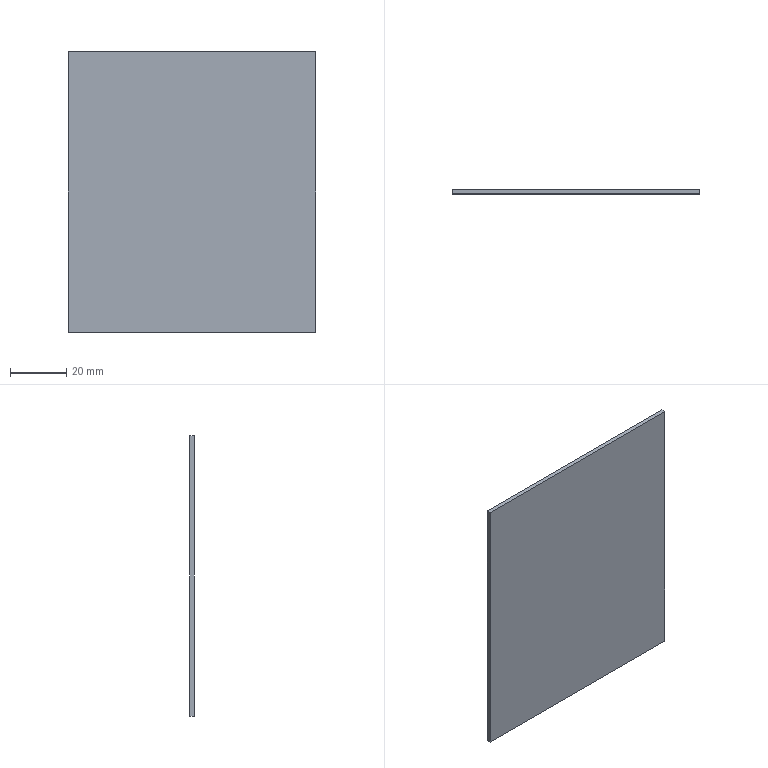Part | STEP file | 1 solid | 6 faces | box 88 x 1.5 x 100 mm | volume 13200 mm3 | plane 6
STEP:
#1=CARTESIAN_POINT('',(0.,0.,0.));
#2=DIRECTION('',(0.,0.,1.));
#3=DIRECTION('',(1.,0.,0.));
#4=AXIS2_PLACEMENT_3D('',#1,#2,#3);
#5=CARTESIAN_POINT('',(44.,0.,50.));
#6=VERTEX_POINT('',#5);
#7=CARTESIAN_POINT('',(44.,0.,-50.));
#8=VERTEX_POINT('',#7);
#9=CARTESIAN_POINT('',(44.,0.,-50.));
#10=DIRECTION('',(0.,0.,-1.));
#11=VECTOR('',#10,1.);
#12=LINE('',#9,#11);
#13=CARTESIAN_POINT('',(44.,1.5,-50.));
#14=DIRECTION('',(-1.,0.,0.));
#15=DIRECTION('',(0.,0.,1.));
#16=AXIS2_PLACEMENT_3D('',#13,#14,#15);
#17=PLANE('',#16);
#18=CARTESIAN_POINT('',(0.,-1.5));
#19=DIRECTION('',(-1.,0.));
#20=VECTOR('',#19,1.);
#21=LINE('',#18,#20);
#22=(GEOMETRIC_REPRESENTATION_CONTEXT(2)PARAMETRIC_REPRESENTATION_CONTEXT()REPRESENTATION_CONTEXT('',''));
#23=DEFINITIONAL_REPRESENTATION('',(#21),#22);
#24=PCURVE('',#17,#23);
#25=CARTESIAN_POINT('',(0.,0.,0.));
#26=DIRECTION('',(0.,1.,0.));
#27=DIRECTION('',(0.,0.,1.));
#28=AXIS2_PLACEMENT_3D('',#25,#26,#27);
#29=PLANE('',#28);
#30=CARTESIAN_POINT('',(-50.,44.));
#31=DIRECTION('',(-1.,0.));
#32=VECTOR('',#31,1.);
#33=LINE('',#30,#32);
#34=(GEOMETRIC_REPRESENTATION_CONTEXT(2)PARAMETRIC_REPRESENTATION_CONTEXT()REPRESENTATION_CONTEXT('',''));
#35=DEFINITIONAL_REPRESENTATION('',(#33),#34);
#36=PCURVE('',#29,#35);
#37=SURFACE_CURVE('',#12,(#24,#36),.PCURVE_S1.);
#38=EDGE_CURVE('',#6,#8,#37,.T.);
#39=ORIENTED_EDGE('',*,*,#38,.T.);
#40=CARTESIAN_POINT('',(44.,1.5,-50.));
#41=VERTEX_POINT('',#40);
#42=CARTESIAN_POINT('',(44.,1.5,-50.));
#43=DIRECTION('',(0.,-1.,0.));
#44=VECTOR('',#43,1.);
#45=LINE('',#42,#44);
#46=CARTESIAN_POINT('',(0.,0.));
#47=DIRECTION('',(0.,-1.));
#48=VECTOR('',#47,1.);
#49=LINE('',#46,#48);
#50=(GEOMETRIC_REPRESENTATION_CONTEXT(2)PARAMETRIC_REPRESENTATION_CONTEXT()REPRESENTATION_CONTEXT('',''));
#51=DEFINITIONAL_REPRESENTATION('',(#49),#50);
#52=PCURVE('',#17,#51);
#53=CARTESIAN_POINT('',(-44.,1.5,-50.));
#54=DIRECTION('',(0.,0.,1.));
#55=DIRECTION('',(1.,0.,0.));
#56=AXIS2_PLACEMENT_3D('',#53,#54,#55);
#57=PLANE('',#56);
#58=CARTESIAN_POINT('',(88.,0.));
#59=DIRECTION('',(0.,-1.));
#60=VECTOR('',#59,1.);
#61=LINE('',#58,#60);
#62=(GEOMETRIC_REPRESENTATION_CONTEXT(2)PARAMETRIC_REPRESENTATION_CONTEXT()REPRESENTATION_CONTEXT('',''));
#63=DEFINITIONAL_REPRESENTATION('',(#61),#62);
#64=PCURVE('',#57,#63);
#65=SURFACE_CURVE('',#45,(#52,#64),.PCURVE_S1.);
#66=EDGE_CURVE('',#41,#8,#65,.T.);
#67=ORIENTED_EDGE('',*,*,#66,.F.);
#68=CARTESIAN_POINT('',(44.,1.5,50.));
#69=VERTEX_POINT('',#68);
#70=CARTESIAN_POINT('',(44.,1.5,-50.));
#71=DIRECTION('',(0.,0.,-1.));
#72=VECTOR('',#71,1.);
#73=LINE('',#70,#72);
#74=CARTESIAN_POINT('',(0.,0.));
#75=DIRECTION('',(-1.,0.));
#76=VECTOR('',#75,1.);
#77=LINE('',#74,#76);
#78=(GEOMETRIC_REPRESENTATION_CONTEXT(2)PARAMETRIC_REPRESENTATION_CONTEXT()REPRESENTATION_CONTEXT('',''));
#79=DEFINITIONAL_REPRESENTATION('',(#77),#78);
#80=PCURVE('',#17,#79);
#81=CARTESIAN_POINT('',(0.,1.5,0.));
#82=DIRECTION('',(0.,1.,0.));
#83=DIRECTION('',(0.,0.,1.));
#84=AXIS2_PLACEMENT_3D('',#81,#82,#83);
#85=PLANE('',#84);
#86=CARTESIAN_POINT('',(-50.,44.));
#87=DIRECTION('',(-1.,0.));
#88=VECTOR('',#87,1.);
#89=LINE('',#86,#88);
#90=(GEOMETRIC_REPRESENTATION_CONTEXT(2)PARAMETRIC_REPRESENTATION_CONTEXT()REPRESENTATION_CONTEXT('',''));
#91=DEFINITIONAL_REPRESENTATION('',(#89),#90);
#92=PCURVE('',#85,#91);
#93=SURFACE_CURVE('',#73,(#80,#92),.PCURVE_S1.);
#94=EDGE_CURVE('',#69,#41,#93,.T.);
#95=ORIENTED_EDGE('',*,*,#94,.F.);
#96=CARTESIAN_POINT('',(44.,1.5,50.));
#97=DIRECTION('',(0.,-1.,0.));
#98=VECTOR('',#97,1.);
#99=LINE('',#96,#98);
#100=CARTESIAN_POINT('',(100.,0.));
#101=DIRECTION('',(0.,-1.));
#102=VECTOR('',#101,1.);
#103=LINE('',#100,#102);
#104=(GEOMETRIC_REPRESENTATION_CONTEXT(2)PARAMETRIC_REPRESENTATION_CONTEXT()REPRESENTATION_CONTEXT('',''));
#105=DEFINITIONAL_REPRESENTATION('',(#103),#104);
#106=PCURVE('',#17,#105);
#107=CARTESIAN_POINT('',(-44.,1.5,50.));
#108=DIRECTION('',(0.,0.,-1.));
#109=DIRECTION('',(-1.,0.,0.));
#110=AXIS2_PLACEMENT_3D('',#107,#108,#109);
#111=PLANE('',#110);
#112=CARTESIAN_POINT('',(-88.,0.));
#113=DIRECTION('',(0.,-1.));
#114=VECTOR('',#113,1.);
#115=LINE('',#112,#114);
#116=(GEOMETRIC_REPRESENTATION_CONTEXT(2)PARAMETRIC_REPRESENTATION_CONTEXT()REPRESENTATION_CONTEXT('',''));
#117=DEFINITIONAL_REPRESENTATION('',(#115),#116);
#118=PCURVE('',#111,#117);
#119=SURFACE_CURVE('',#99,(#106,#118),.PCURVE_S1.);
#120=EDGE_CURVE('',#69,#6,#119,.T.);
#121=ORIENTED_EDGE('',*,*,#120,.T.);
#122=EDGE_LOOP('',(#39,#67,#95,#121));
#123=FACE_BOUND('',#122,.T.);
#124=ADVANCED_FACE('',(#123),#17,.F.);
#125=CARTESIAN_POINT('',(-44.,0.,-50.));
#126=VERTEX_POINT('',#125);
#127=CARTESIAN_POINT('',(-44.,0.,-50.));
#128=DIRECTION('',(-1.,0.,0.));
#129=VECTOR('',#128,1.);
#130=LINE('',#127,#129);
#131=CARTESIAN_POINT('',(0.,-1.5));
#132=DIRECTION('',(-1.,0.));
#133=VECTOR('',#132,1.);
#134=LINE('',#131,#133);
#135=(GEOMETRIC_REPRESENTATION_CONTEXT(2)PARAMETRIC_REPRESENTATION_CONTEXT()REPRESENTATION_CONTEXT('',''));
#136=DEFINITIONAL_REPRESENTATION('',(#134),#135);
#137=PCURVE('',#57,#136);
#138=CARTESIAN_POINT('',(-50.,-44.));
#139=DIRECTION('',(0.,-1.));
#140=VECTOR('',#139,1.);
#141=LINE('',#138,#140);
#142=(GEOMETRIC_REPRESENTATION_CONTEXT(2)PARAMETRIC_REPRESENTATION_CONTEXT()REPRESENTATION_CONTEXT('',''));
#143=DEFINITIONAL_REPRESENTATION('',(#141),#142);
#144=PCURVE('',#29,#143);
#145=SURFACE_CURVE('',#130,(#137,#144),.PCURVE_S1.);
#146=EDGE_CURVE('',#8,#126,#145,.T.);
#147=ORIENTED_EDGE('',*,*,#146,.T.);
#148=CARTESIAN_POINT('',(-44.,1.5,-50.));
#149=VERTEX_POINT('',#148);
#150=CARTESIAN_POINT('',(-44.,1.5,-50.));
#151=DIRECTION('',(0.,-1.,0.));
#152=VECTOR('',#151,1.);
#153=LINE('',#150,#152);
#154=CARTESIAN_POINT('',(0.,0.));
#155=DIRECTION('',(0.,-1.));
#156=VECTOR('',#155,1.);
#157=LINE('',#154,#156);
#158=(GEOMETRIC_REPRESENTATION_CONTEXT(2)PARAMETRIC_REPRESENTATION_CONTEXT()REPRESENTATION_CONTEXT('',''));
#159=DEFINITIONAL_REPRESENTATION('',(#157),#158);
#160=PCURVE('',#57,#159);
#161=CARTESIAN_POINT('',(-44.,1.5,-50.));
#162=DIRECTION('',(1.,0.,0.));
#163=DIRECTION('',(0.,0.,-1.));
#164=AXIS2_PLACEMENT_3D('',#161,#162,#163);
#165=PLANE('',#164);
#166=CARTESIAN_POINT('',(0.,0.));
#167=DIRECTION('',(0.,-1.));
#168=VECTOR('',#167,1.);
#169=LINE('',#166,#168);
#170=(GEOMETRIC_REPRESENTATION_CONTEXT(2)PARAMETRIC_REPRESENTATION_CONTEXT()REPRESENTATION_CONTEXT('',''));
#171=DEFINITIONAL_REPRESENTATION('',(#169),#170);
#172=PCURVE('',#165,#171);
#173=SURFACE_CURVE('',#153,(#160,#172),.PCURVE_S1.);
#174=EDGE_CURVE('',#149,#126,#173,.T.);
#175=ORIENTED_EDGE('',*,*,#174,.F.);
#176=CARTESIAN_POINT('',(-44.,1.5,-50.));
#177=DIRECTION('',(-1.,0.,0.));
#178=VECTOR('',#177,1.);
#179=LINE('',#176,#178);
#180=CARTESIAN_POINT('',(0.,0.));
#181=DIRECTION('',(-1.,0.));
#182=VECTOR('',#181,1.);
#183=LINE('',#180,#182);
#184=(GEOMETRIC_REPRESENTATION_CONTEXT(2)PARAMETRIC_REPRESENTATION_CONTEXT()REPRESENTATION_CONTEXT('',''));
#185=DEFINITIONAL_REPRESENTATION('',(#183),#184);
#186=PCURVE('',#57,#185);
#187=CARTESIAN_POINT('',(-50.,-44.));
#188=DIRECTION('',(0.,-1.));
#189=VECTOR('',#188,1.);
#190=LINE('',#187,#189);
#191=(GEOMETRIC_REPRESENTATION_CONTEXT(2)PARAMETRIC_REPRESENTATION_CONTEXT()REPRESENTATION_CONTEXT('',''));
#192=DEFINITIONAL_REPRESENTATION('',(#190),#191);
#193=PCURVE('',#85,#192);
#194=SURFACE_CURVE('',#179,(#186,#193),.PCURVE_S1.);
#195=EDGE_CURVE('',#41,#149,#194,.T.);
#196=ORIENTED_EDGE('',*,*,#195,.F.);
#197=ORIENTED_EDGE('',*,*,#66,.T.);
#198=EDGE_LOOP('',(#147,#175,#196,#197));
#199=FACE_BOUND('',#198,.T.);
#200=ADVANCED_FACE('',(#199),#57,.F.);
#201=CARTESIAN_POINT('',(-44.,0.,50.));
#202=VERTEX_POINT('',#201);
#203=CARTESIAN_POINT('',(-44.,0.,-50.));
#204=DIRECTION('',(0.,0.,1.));
#205=VECTOR('',#204,1.);
#206=LINE('',#203,#205);
#207=CARTESIAN_POINT('',(0.,-1.5));
#208=DIRECTION('',(-1.,0.));
#209=VECTOR('',#208,1.);
#210=LINE('',#207,#209);
#211=(GEOMETRIC_REPRESENTATION_CONTEXT(2)PARAMETRIC_REPRESENTATION_CONTEXT()REPRESENTATION_CONTEXT('',''));
#212=DEFINITIONAL_REPRESENTATION('',(#210),#211);
#213=PCURVE('',#165,#212);
#214=CARTESIAN_POINT('',(-50.,-44.));
#215=DIRECTION('',(1.,0.));
#216=VECTOR('',#215,1.);
#217=LINE('',#214,#216);
#218=(GEOMETRIC_REPRESENTATION_CONTEXT(2)PARAMETRIC_REPRESENTATION_CONTEXT()REPRESENTATION_CONTEXT('',''));
#219=DEFINITIONAL_REPRESENTATION('',(#217),#218);
#220=PCURVE('',#29,#219);
#221=SURFACE_CURVE('',#206,(#213,#220),.PCURVE_S1.);
#222=EDGE_CURVE('',#126,#202,#221,.T.);
#223=ORIENTED_EDGE('',*,*,#222,.T.);
#224=CARTESIAN_POINT('',(-44.,1.5,50.));
#225=VERTEX_POINT('',#224);
#226=CARTESIAN_POINT('',(-44.,1.5,50.));
#227=DIRECTION('',(0.,-1.,0.));
#228=VECTOR('',#227,1.);
#229=LINE('',#226,#228);
#230=CARTESIAN_POINT('',(-100.,0.));
#231=DIRECTION('',(0.,-1.));
#232=VECTOR('',#231,1.);
#233=LINE('',#230,#232);
#234=(GEOMETRIC_REPRESENTATION_CONTEXT(2)PARAMETRIC_REPRESENTATION_CONTEXT()REPRESENTATION_CONTEXT('',''));
#235=DEFINITIONAL_REPRESENTATION('',(#233),#234);
#236=PCURVE('',#165,#235);
#237=CARTESIAN_POINT('',(0.,0.));
#238=DIRECTION('',(0.,-1.));
#239=VECTOR('',#238,1.);
#240=LINE('',#237,#239);
#241=(GEOMETRIC_REPRESENTATION_CONTEXT(2)PARAMETRIC_REPRESENTATION_CONTEXT()REPRESENTATION_CONTEXT('',''));
#242=DEFINITIONAL_REPRESENTATION('',(#240),#241);
#243=PCURVE('',#111,#242);
#244=SURFACE_CURVE('',#229,(#236,#243),.PCURVE_S1.);
#245=EDGE_CURVE('',#225,#202,#244,.T.);
#246=ORIENTED_EDGE('',*,*,#245,.F.);
#247=CARTESIAN_POINT('',(-44.,1.5,-50.));
#248=DIRECTION('',(0.,0.,1.));
#249=VECTOR('',#248,1.);
#250=LINE('',#247,#249);
#251=CARTESIAN_POINT('',(0.,0.));
#252=DIRECTION('',(-1.,0.));
#253=VECTOR('',#252,1.);
#254=LINE('',#251,#253);
#255=(GEOMETRIC_REPRESENTATION_CONTEXT(2)PARAMETRIC_REPRESENTATION_CONTEXT()REPRESENTATION_CONTEXT('',''));
#256=DEFINITIONAL_REPRESENTATION('',(#254),#255);
#257=PCURVE('',#165,#256);
#258=CARTESIAN_POINT('',(-50.,-44.));
#259=DIRECTION('',(1.,0.));
#260=VECTOR('',#259,1.);
#261=LINE('',#258,#260);
#262=(GEOMETRIC_REPRESENTATION_CONTEXT(2)PARAMETRIC_REPRESENTATION_CONTEXT()REPRESENTATION_CONTEXT('',''));
#263=DEFINITIONAL_REPRESENTATION('',(#261),#262);
#264=PCURVE('',#85,#263);
#265=SURFACE_CURVE('',#250,(#257,#264),.PCURVE_S1.);
#266=EDGE_CURVE('',#149,#225,#265,.T.);
#267=ORIENTED_EDGE('',*,*,#266,.F.);
#268=ORIENTED_EDGE('',*,*,#174,.T.);
#269=EDGE_LOOP('',(#223,#246,#267,#268));
#270=FACE_BOUND('',#269,.T.);
#271=ADVANCED_FACE('',(#270),#165,.F.);
#272=CARTESIAN_POINT('',(-44.,0.,50.));
#273=DIRECTION('',(1.,0.,0.));
#274=VECTOR('',#273,1.);
#275=LINE('',#272,#274);
#276=CARTESIAN_POINT('',(0.,-1.5));
#277=DIRECTION('',(-1.,0.));
#278=VECTOR('',#277,1.);
#279=LINE('',#276,#278);
#280=(GEOMETRIC_REPRESENTATION_CONTEXT(2)PARAMETRIC_REPRESENTATION_CONTEXT()REPRESENTATION_CONTEXT('',''));
#281=DEFINITIONAL_REPRESENTATION('',(#279),#280);
#282=PCURVE('',#111,#281);
#283=CARTESIAN_POINT('',(50.,-44.));
#284=DIRECTION('',(0.,1.));
#285=VECTOR('',#284,1.);
#286=LINE('',#283,#285);
#287=(GEOMETRIC_REPRESENTATION_CONTEXT(2)PARAMETRIC_REPRESENTATION_CONTEXT()REPRESENTATION_CONTEXT('',''));
#288=DEFINITIONAL_REPRESENTATION('',(#286),#287);
#289=PCURVE('',#29,#288);
#290=SURFACE_CURVE('',#275,(#282,#289),.PCURVE_S1.);
#291=EDGE_CURVE('',#202,#6,#290,.T.);
#292=ORIENTED_EDGE('',*,*,#291,.T.);
#293=ORIENTED_EDGE('',*,*,#120,.F.);
#294=CARTESIAN_POINT('',(-44.,1.5,50.));
#295=DIRECTION('',(1.,0.,0.));
#296=VECTOR('',#295,1.);
#297=LINE('',#294,#296);
#298=CARTESIAN_POINT('',(0.,0.));
#299=DIRECTION('',(-1.,0.));
#300=VECTOR('',#299,1.);
#301=LINE('',#298,#300);
#302=(GEOMETRIC_REPRESENTATION_CONTEXT(2)PARAMETRIC_REPRESENTATION_CONTEXT()REPRESENTATION_CONTEXT('',''));
#303=DEFINITIONAL_REPRESENTATION('',(#301),#302);
#304=PCURVE('',#111,#303);
#305=CARTESIAN_POINT('',(50.,-44.));
#306=DIRECTION('',(0.,1.));
#307=VECTOR('',#306,1.);
#308=LINE('',#305,#307);
#309=(GEOMETRIC_REPRESENTATION_CONTEXT(2)PARAMETRIC_REPRESENTATION_CONTEXT()REPRESENTATION_CONTEXT('',''));
#310=DEFINITIONAL_REPRESENTATION('',(#308),#309);
#311=PCURVE('',#85,#310);
#312=SURFACE_CURVE('',#297,(#304,#311),.PCURVE_S1.);
#313=EDGE_CURVE('',#225,#69,#312,.T.);
#314=ORIENTED_EDGE('',*,*,#313,.F.);
#315=ORIENTED_EDGE('',*,*,#245,.T.);
#316=EDGE_LOOP('',(#292,#293,#314,#315));
#317=FACE_BOUND('',#316,.T.);
#318=ADVANCED_FACE('',(#317),#111,.F.);
#319=ORIENTED_EDGE('',*,*,#94,.T.);
#320=ORIENTED_EDGE('',*,*,#195,.T.);
#321=ORIENTED_EDGE('',*,*,#266,.T.);
#322=ORIENTED_EDGE('',*,*,#313,.T.);
#323=EDGE_LOOP('',(#319,#320,#321,#322));
#324=FACE_BOUND('',#323,.T.);
#325=ADVANCED_FACE('',(#324),#85,.T.);
#326=ORIENTED_EDGE('',*,*,#38,.F.);
#327=ORIENTED_EDGE('',*,*,#291,.F.);
#328=ORIENTED_EDGE('',*,*,#222,.F.);
#329=ORIENTED_EDGE('',*,*,#146,.F.);
#330=EDGE_LOOP('',(#326,#327,#328,#329));
#331=FACE_BOUND('',#330,.T.);
#332=ADVANCED_FACE('',(#331),#29,.F.);
#333=CLOSED_SHELL('',(#124,#200,#271,#318,#325,#332));
#334=MANIFOLD_SOLID_BREP('',#333);
#335=(LENGTH_UNIT()NAMED_UNIT(*)SI_UNIT(.MILLI.,.METRE.));
#336=UNCERTAINTY_MEASURE_WITH_UNIT(LENGTH_MEASURE(0.0000001),#335,'','');
#337=(NAMED_UNIT(*)PLANE_ANGLE_UNIT()SI_UNIT($,.RADIAN.));
#338=(NAMED_UNIT(*)SI_UNIT($,.STERADIAN.)SOLID_ANGLE_UNIT());
#339=(GEOMETRIC_REPRESENTATION_CONTEXT(3)GLOBAL_UNCERTAINTY_ASSIGNED_CONTEXT((#336))GLOBAL_UNIT_ASSIGNED_CONTEXT((#335,#337,#338))REPRESENTATION_CONTEXT('',''));
#340=ADVANCED_BREP_SHAPE_REPRESENTATION('',(#4,#334),#339);